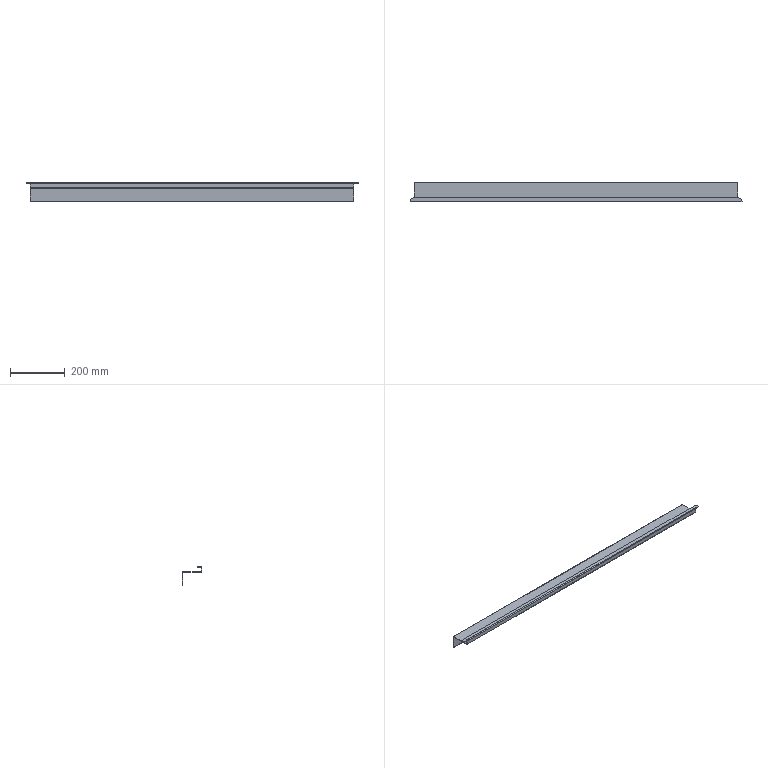Part | SolidWorks | features BaseBody 1 | 1 solid | 36 faces | box 1216 x 72 x 68 mm | volume 352774 mm3 | plane 24 | cylinder 8 | torus 4 | commonest cylinder face diameters 2 x3 6 x3 30 x2
STEP:
#1=CARTESIAN_POINT('',(596.,-36.,18.));
#2=VERTEX_POINT('',#1);
#3=CARTESIAN_POINT('',(593.,-36.,15.));
#4=VERTEX_POINT('',#3);
#5=CARTESIAN_POINT('',(596.,-36.,15.));
#6=DIRECTION('',(0.,-1.,0.));
#7=DIRECTION('',(0.,0.,1.));
#8=AXIS2_PLACEMENT_3D('',#5,#6,#7);
#9=CIRCLE('',#8,3.);
#10=EDGE_CURVE('',#2,#4,#9,.T.);
#11=ORIENTED_EDGE('',*,*,#10,.T.);
#12=CARTESIAN_POINT('',(595.,-36.,15.));
#13=VERTEX_POINT('',#12);
#14=CARTESIAN_POINT('',(595.,-36.,15.));
#15=DIRECTION('',(1.,0.,0.));
#16=VECTOR('',#15,1000.);
#17=LINE('',#14,#16);
#18=EDGE_CURVE('',#4,#13,#17,.T.);
#19=ORIENTED_EDGE('',*,*,#18,.T.);
#20=CARTESIAN_POINT('',(596.,-36.,16.));
#21=VERTEX_POINT('',#20);
#22=CARTESIAN_POINT('',(596.,-36.,15.));
#23=DIRECTION('',(0.,1.,0.));
#24=DIRECTION('',(0.,0.,1.));
#25=AXIS2_PLACEMENT_3D('',#22,#23,#24);
#26=CIRCLE('',#25,1.);
#27=EDGE_CURVE('',#13,#21,#26,.T.);
#28=ORIENTED_EDGE('',*,*,#27,.T.);
#29=CARTESIAN_POINT('',(608.,-36.,16.));
#30=VERTEX_POINT('',#29);
#31=CARTESIAN_POINT('',(608.,-36.,16.));
#32=DIRECTION('',(1.,0.,0.));
#33=VECTOR('',#32,1000.);
#34=LINE('',#31,#33);
#35=EDGE_CURVE('',#21,#30,#34,.T.);
#36=ORIENTED_EDGE('',*,*,#35,.T.);
#37=CARTESIAN_POINT('',(608.,-36.,18.));
#38=VERTEX_POINT('',#37);
#39=CARTESIAN_POINT('',(608.,-36.,18.));
#40=DIRECTION('',(0.,0.,1.));
#41=VECTOR('',#40,1000.);
#42=LINE('',#39,#41);
#43=EDGE_CURVE('',#30,#38,#42,.T.);
#44=ORIENTED_EDGE('',*,*,#43,.T.);
#45=CARTESIAN_POINT('',(596.,-36.,18.));
#46=DIRECTION('',(-1.,0.,0.));
#47=VECTOR('',#46,1000.);
#48=LINE('',#45,#47);
#49=EDGE_CURVE('',#38,#2,#48,.T.);
#50=ORIENTED_EDGE('',*,*,#49,.T.);
#51=EDGE_LOOP('',(#11,#19,#28,#36,#44,#50));
#52=FACE_OUTER_BOUND('',#51,.T.);
#53=CARTESIAN_POINT('',(596.,-36.,15.));
#54=DIRECTION('',(0.,-1.,0.));
#55=DIRECTION('',(0.,0.,-1.));
#56=AXIS2_PLACEMENT_3D('',#53,#54,#55);
#57=PLANE('',#56);
#58=ADVANCED_FACE('',(#52),#57,.T.);
#59=CARTESIAN_POINT('',(593.,-33.,16.));
#60=VERTEX_POINT('',#59);
#61=CARTESIAN_POINT('',(593.,-36.,16.));
#62=DIRECTION('',(0.,0.,-1.));
#63=DIRECTION('',(0.,1.,0.));
#64=AXIS2_PLACEMENT_3D('',#61,#62,#63);
#65=CIRCLE('',#64,3.);
#66=EDGE_CURVE('',#60,#21,#65,.T.);
#67=ORIENTED_EDGE('',*,*,#66,.T.);
#68=ORIENTED_EDGE('',*,*,#27,.F.);
#69=CARTESIAN_POINT('',(593.,-34.,15.));
#70=VERTEX_POINT('',#69);
#71=CARTESIAN_POINT('',(593.,-36.,15.));
#72=DIRECTION('',(0.,0.,-1.));
#73=DIRECTION('',(0.,1.,0.));
#74=AXIS2_PLACEMENT_3D('',#71,#72,#73);
#75=CIRCLE('',#74,2.);
#76=EDGE_CURVE('',#70,#13,#75,.T.);
#77=ORIENTED_EDGE('',*,*,#76,.F.);
#78=CARTESIAN_POINT('',(593.,-33.,15.));
#79=DIRECTION('',(1.,0.,0.));
#80=DIRECTION('',(0.,0.,-1.));
#81=AXIS2_PLACEMENT_3D('',#78,#79,#80);
#82=CIRCLE('',#81,1.);
#83=EDGE_CURVE('',#60,#70,#82,.T.);
#84=ORIENTED_EDGE('',*,*,#83,.F.);
#85=EDGE_LOOP('',(#67,#68,#77,#84));
#86=FACE_OUTER_BOUND('',#85,.T.);
#87=CARTESIAN_POINT('',(593.,-36.,15.));
#88=DIRECTION('',(0.,0.,-1.));
#89=DIRECTION('',(-1.,0.,0.));
#90=AXIS2_PLACEMENT_3D('',#87,#88,#89);
#91=TOROIDAL_SURFACE('',#90,3.,1.);
#92=ADVANCED_FACE('',(#86),#91,.F.);
#93=CARTESIAN_POINT('',(593.,-21.,18.));
#94=VERTEX_POINT('',#93);
#95=CARTESIAN_POINT('',(593.,-36.,18.));
#96=DIRECTION('',(0.,0.,-1.));
#97=DIRECTION('',(0.,1.,0.));
#98=AXIS2_PLACEMENT_3D('',#95,#96,#97);
#99=CIRCLE('',#98,15.);
#100=EDGE_CURVE('',#94,#38,#99,.T.);
#101=ORIENTED_EDGE('',*,*,#100,.T.);
#102=ORIENTED_EDGE('',*,*,#43,.F.);
#103=CARTESIAN_POINT('',(593.,-21.,16.));
#104=VERTEX_POINT('',#103);
#105=CARTESIAN_POINT('',(593.,-36.,16.));
#106=DIRECTION('',(0.,0.,-1.));
#107=DIRECTION('',(0.,1.,0.));
#108=AXIS2_PLACEMENT_3D('',#105,#106,#107);
#109=CIRCLE('',#108,15.);
#110=EDGE_CURVE('',#104,#30,#109,.T.);
#111=ORIENTED_EDGE('',*,*,#110,.F.);
#112=CARTESIAN_POINT('',(593.,-21.,18.));
#113=DIRECTION('',(0.,0.,-1.));
#114=VECTOR('',#113,1000.);
#115=LINE('',#112,#114);
#116=EDGE_CURVE('',#94,#104,#115,.T.);
#117=ORIENTED_EDGE('',*,*,#116,.F.);
#118=EDGE_LOOP('',(#101,#102,#111,#117));
#119=FACE_OUTER_BOUND('',#118,.T.);
#120=CARTESIAN_POINT('',(593.,-36.,18.));
#121=DIRECTION('',(0.,0.,-1.));
#122=DIRECTION('',(-1.,0.,0.));
#123=AXIS2_PLACEMENT_3D('',#120,#121,#122);
#124=CYLINDRICAL_SURFACE('',#123,15.);
#125=ADVANCED_FACE('',(#119),#124,.T.);
#126=CARTESIAN_POINT('',(593.,-33.,18.));
#127=VERTEX_POINT('',#126);
#128=CARTESIAN_POINT('',(593.,-33.,15.));
#129=DIRECTION('',(1.,0.,0.));
#130=DIRECTION('',(0.,0.,-1.));
#131=AXIS2_PLACEMENT_3D('',#128,#129,#130);
#132=CIRCLE('',#131,3.);
#133=EDGE_CURVE('',#127,#4,#132,.T.);
#134=ORIENTED_EDGE('',*,*,#133,.T.);
#135=ORIENTED_EDGE('',*,*,#10,.F.);
#136=CARTESIAN_POINT('',(593.,-36.,18.));
#137=DIRECTION('',(0.,0.,-1.));
#138=DIRECTION('',(0.,1.,0.));
#139=AXIS2_PLACEMENT_3D('',#136,#137,#138);
#140=CIRCLE('',#139,3.);
#141=EDGE_CURVE('',#127,#2,#140,.T.);
#142=ORIENTED_EDGE('',*,*,#141,.F.);
#143=EDGE_LOOP('',(#134,#135,#142));
#144=FACE_OUTER_BOUND('',#143,.T.);
#145=CARTESIAN_POINT('',(593.,-36.,15.));
#146=DIRECTION('',(0.,0.,-1.));
#147=DIRECTION('',(-1.,0.,0.));
#148=AXIS2_PLACEMENT_3D('',#145,#146,#147);
#149=TOROIDAL_SURFACE('',#148,3.,3.);
#150=ADVANCED_FACE('',(#144),#149,.T.);
#151=ORIENTED_EDGE('',*,*,#18,.F.);
#152=CARTESIAN_POINT('',(593.,-34.,15.));
#153=DIRECTION('',(0.,-1.,0.));
#154=VECTOR('',#153,1000.);
#155=LINE('',#152,#154);
#156=EDGE_CURVE('',#70,#4,#155,.T.);
#157=ORIENTED_EDGE('',*,*,#156,.F.);
#158=ORIENTED_EDGE('',*,*,#76,.T.);
#159=EDGE_LOOP('',(#151,#157,#158));
#160=FACE_OUTER_BOUND('',#159,.T.);
#161=CARTESIAN_POINT('',(593.,-34.,15.));
#162=DIRECTION('',(0.,0.,-1.));
#163=DIRECTION('',(0.,-1.,0.));
#164=AXIS2_PLACEMENT_3D('',#161,#162,#163);
#165=PLANE('',#164);
#166=ADVANCED_FACE('',(#160),#165,.T.);
#167=CARTESIAN_POINT('',(-593.,-36.,15.));
#168=VERTEX_POINT('',#167);
#169=CARTESIAN_POINT('',(-596.,-36.,18.));
#170=VERTEX_POINT('',#169);
#171=CARTESIAN_POINT('',(-596.,-36.,15.));
#172=DIRECTION('',(0.,-1.,0.));
#173=DIRECTION('',(0.,0.,1.));
#174=AXIS2_PLACEMENT_3D('',#171,#172,#173);
#175=CIRCLE('',#174,3.);
#176=EDGE_CURVE('',#168,#170,#175,.T.);
#177=ORIENTED_EDGE('',*,*,#176,.T.);
#178=CARTESIAN_POINT('',(-608.,-36.,18.));
#179=VERTEX_POINT('',#178);
#180=CARTESIAN_POINT('',(-596.,-36.,18.));
#181=DIRECTION('',(-1.,0.,0.));
#182=VECTOR('',#181,1000.);
#183=LINE('',#180,#182);
#184=EDGE_CURVE('',#170,#179,#183,.T.);
#185=ORIENTED_EDGE('',*,*,#184,.T.);
#186=CARTESIAN_POINT('',(-608.,-36.,16.));
#187=VERTEX_POINT('',#186);
#188=CARTESIAN_POINT('',(-608.,-36.,18.));
#189=DIRECTION('',(0.,0.,-1.));
#190=VECTOR('',#189,1000.);
#191=LINE('',#188,#190);
#192=EDGE_CURVE('',#179,#187,#191,.T.);
#193=ORIENTED_EDGE('',*,*,#192,.T.);
#194=CARTESIAN_POINT('',(-596.,-36.,16.));
#195=VERTEX_POINT('',#194);
#196=CARTESIAN_POINT('',(-608.,-36.,16.));
#197=DIRECTION('',(1.,0.,0.));
#198=VECTOR('',#197,1000.);
#199=LINE('',#196,#198);
#200=EDGE_CURVE('',#187,#195,#199,.T.);
#201=ORIENTED_EDGE('',*,*,#200,.T.);
#202=CARTESIAN_POINT('',(-595.,-36.,15.));
#203=VERTEX_POINT('',#202);
#204=CARTESIAN_POINT('',(-596.,-36.,15.));
#205=DIRECTION('',(0.,1.,0.));
#206=DIRECTION('',(0.,0.,1.));
#207=AXIS2_PLACEMENT_3D('',#204,#205,#206);
#208=CIRCLE('',#207,1.);
#209=EDGE_CURVE('',#195,#203,#208,.T.);
#210=ORIENTED_EDGE('',*,*,#209,.T.);
#211=CARTESIAN_POINT('',(-595.,-36.,15.));
#212=DIRECTION('',(1.,0.,0.));
#213=VECTOR('',#212,1000.);
#214=LINE('',#211,#213);
#215=EDGE_CURVE('',#203,#168,#214,.T.);
#216=ORIENTED_EDGE('',*,*,#215,.T.);
#217=EDGE_LOOP('',(#177,#185,#193,#201,#210,#216));
#218=FACE_OUTER_BOUND('',#217,.T.);
#219=CARTESIAN_POINT('',(-596.,-36.,15.));
#220=DIRECTION('',(0.,-1.,0.));
#221=DIRECTION('',(0.,0.,-1.));
#222=AXIS2_PLACEMENT_3D('',#219,#220,#221);
#223=PLANE('',#222);
#224=ADVANCED_FACE('',(#218),#223,.T.);
#225=CARTESIAN_POINT('',(-593.,-33.,18.));
#226=VERTEX_POINT('',#225);
#227=CARTESIAN_POINT('',(-593.,-36.,18.));
#228=DIRECTION('',(0.,0.,1.));
#229=DIRECTION('',(0.,1.,0.));
#230=AXIS2_PLACEMENT_3D('',#227,#228,#229);
#231=CIRCLE('',#230,3.);
#232=EDGE_CURVE('',#226,#170,#231,.T.);
#233=ORIENTED_EDGE('',*,*,#232,.T.);
#234=ORIENTED_EDGE('',*,*,#176,.F.);
#235=CARTESIAN_POINT('',(-593.,-33.,15.));
#236=DIRECTION('',(-1.,0.,0.));
#237=DIRECTION('',(0.,0.,-1.));
#238=AXIS2_PLACEMENT_3D('',#235,#236,#237);
#239=CIRCLE('',#238,3.);
#240=EDGE_CURVE('',#168,#226,#239,.T.);
#241=ORIENTED_EDGE('',*,*,#240,.T.);
#242=EDGE_LOOP('',(#233,#234,#241));
#243=FACE_OUTER_BOUND('',#242,.T.);
#244=CARTESIAN_POINT('',(-593.,-36.,15.));
#245=DIRECTION('',(0.,0.,1.));
#246=DIRECTION('',(1.,0.,0.));
#247=AXIS2_PLACEMENT_3D('',#244,#245,#246);
#248=TOROIDAL_SURFACE('',#247,3.,3.);
#249=ADVANCED_FACE('',(#243),#248,.T.);
#250=CARTESIAN_POINT('',(-593.,-21.,16.));
#251=VERTEX_POINT('',#250);
#252=CARTESIAN_POINT('',(-593.,-36.,16.));
#253=DIRECTION('',(0.,0.,1.));
#254=DIRECTION('',(0.,1.,0.));
#255=AXIS2_PLACEMENT_3D('',#252,#253,#254);
#256=CIRCLE('',#255,15.);
#257=EDGE_CURVE('',#251,#187,#256,.T.);
#258=ORIENTED_EDGE('',*,*,#257,.T.);
#259=ORIENTED_EDGE('',*,*,#192,.F.);
#260=CARTESIAN_POINT('',(-593.,-21.,18.));
#261=VERTEX_POINT('',#260);
#262=CARTESIAN_POINT('',(-593.,-36.,18.));
#263=DIRECTION('',(0.,0.,1.));
#264=DIRECTION('',(0.,1.,0.));
#265=AXIS2_PLACEMENT_3D('',#262,#263,#264);
#266=CIRCLE('',#265,15.);
#267=EDGE_CURVE('',#261,#179,#266,.T.);
#268=ORIENTED_EDGE('',*,*,#267,.F.);
#269=CARTESIAN_POINT('',(-593.,-21.,18.));
#270=DIRECTION('',(0.,0.,-1.));
#271=VECTOR('',#270,1000.);
#272=LINE('',#269,#271);
#273=EDGE_CURVE('',#261,#251,#272,.T.);
#274=ORIENTED_EDGE('',*,*,#273,.T.);
#275=EDGE_LOOP('',(#258,#259,#268,#274));
#276=FACE_OUTER_BOUND('',#275,.T.);
#277=CARTESIAN_POINT('',(-593.,-36.,18.));
#278=DIRECTION('',(0.,0.,1.));
#279=DIRECTION('',(1.,0.,0.));
#280=AXIS2_PLACEMENT_3D('',#277,#278,#279);
#281=CYLINDRICAL_SURFACE('',#280,15.);
#282=ADVANCED_FACE('',(#276),#281,.T.);
#283=CARTESIAN_POINT('',(-593.,-34.,15.));
#284=VERTEX_POINT('',#283);
#285=CARTESIAN_POINT('',(-593.,-36.,15.));
#286=DIRECTION('',(0.,0.,1.));
#287=DIRECTION('',(0.,1.,0.));
#288=AXIS2_PLACEMENT_3D('',#285,#286,#287);
#289=CIRCLE('',#288,2.);
#290=EDGE_CURVE('',#284,#203,#289,.T.);
#291=ORIENTED_EDGE('',*,*,#290,.T.);
#292=ORIENTED_EDGE('',*,*,#209,.F.);
#293=CARTESIAN_POINT('',(-593.,-33.,16.));
#294=VERTEX_POINT('',#293);
#295=CARTESIAN_POINT('',(-593.,-36.,16.));
#296=DIRECTION('',(0.,0.,1.));
#297=DIRECTION('',(0.,1.,0.));
#298=AXIS2_PLACEMENT_3D('',#295,#296,#297);
#299=CIRCLE('',#298,3.);
#300=EDGE_CURVE('',#294,#195,#299,.T.);
#301=ORIENTED_EDGE('',*,*,#300,.F.);
#302=CARTESIAN_POINT('',(-593.,-33.,15.));
#303=DIRECTION('',(-1.,0.,0.));
#304=DIRECTION('',(0.,0.,-1.));
#305=AXIS2_PLACEMENT_3D('',#302,#303,#304);
#306=CIRCLE('',#305,1.);
#307=EDGE_CURVE('',#284,#294,#306,.T.);
#308=ORIENTED_EDGE('',*,*,#307,.F.);
#309=EDGE_LOOP('',(#291,#292,#301,#308));
#310=FACE_OUTER_BOUND('',#309,.T.);
#311=CARTESIAN_POINT('',(-593.,-36.,15.));
#312=DIRECTION('',(0.,0.,1.));
#313=DIRECTION('',(1.,0.,0.));
#314=AXIS2_PLACEMENT_3D('',#311,#312,#313);
#315=TOROIDAL_SURFACE('',#314,3.,1.);
#316=ADVANCED_FACE('',(#310),#315,.F.);
#317=ORIENTED_EDGE('',*,*,#215,.F.);
#318=ORIENTED_EDGE('',*,*,#290,.F.);
#319=CARTESIAN_POINT('',(-593.,-34.,15.));
#320=DIRECTION('',(0.,-1.,0.));
#321=VECTOR('',#320,1000.);
#322=LINE('',#319,#321);
#323=EDGE_CURVE('',#284,#168,#322,.T.);
#324=ORIENTED_EDGE('',*,*,#323,.T.);
#325=EDGE_LOOP('',(#317,#318,#324));
#326=FACE_OUTER_BOUND('',#325,.T.);
#327=CARTESIAN_POINT('',(-593.,-34.,15.));
#328=DIRECTION('',(0.,0.,-1.));
#329=DIRECTION('',(0.,-1.,0.));
#330=AXIS2_PLACEMENT_3D('',#327,#328,#329);
#331=PLANE('',#330);
#332=ADVANCED_FACE('',(#326),#331,.T.);
#333=CARTESIAN_POINT('',(-593.,-21.,16.));
#334=DIRECTION('',(-1.,0.,0.));
#335=VECTOR('',#334,1000.);
#336=LINE('',#333,#335);
#337=EDGE_CURVE('',#104,#251,#336,.T.);
#338=ORIENTED_EDGE('',*,*,#337,.T.);
#339=ORIENTED_EDGE('',*,*,#273,.F.);
#340=CARTESIAN_POINT('',(0.,-21.,18.));
#341=DIRECTION('',(-1.,0.,0.));
#342=VECTOR('',#341,1000.);
#343=LINE('',#340,#342);
#344=EDGE_CURVE('',#94,#261,#343,.T.);
#345=ORIENTED_EDGE('',*,*,#344,.F.);
#346=ORIENTED_EDGE('',*,*,#116,.T.);
#347=EDGE_LOOP('',(#338,#339,#345,#346));
#348=FACE_OUTER_BOUND('',#347,.T.);
#349=CARTESIAN_POINT('',(-593.,-21.,18.));
#350=DIRECTION('',(0.,-1.,0.));
#351=DIRECTION('',(0.,0.,-1.));
#352=AXIS2_PLACEMENT_3D('',#349,#350,#351);
#353=PLANE('',#352);
#354=ADVANCED_FACE('',(#348),#353,.F.);
#355=ORIENTED_EDGE('',*,*,#337,.F.);
#356=ORIENTED_EDGE('',*,*,#110,.T.);
#357=ORIENTED_EDGE('',*,*,#35,.F.);
#358=ORIENTED_EDGE('',*,*,#66,.F.);
#359=CARTESIAN_POINT('',(-593.,-33.,16.));
#360=DIRECTION('',(1.,0.,0.));
#361=VECTOR('',#360,1000.);
#362=LINE('',#359,#361);
#363=EDGE_CURVE('',#294,#60,#362,.T.);
#364=ORIENTED_EDGE('',*,*,#363,.F.);
#365=ORIENTED_EDGE('',*,*,#300,.T.);
#366=ORIENTED_EDGE('',*,*,#200,.F.);
#367=ORIENTED_EDGE('',*,*,#257,.F.);
#368=EDGE_LOOP('',(#355,#356,#357,#358,#364,#365,#366,#367));
#369=FACE_OUTER_BOUND('',#368,.T.);
#370=CARTESIAN_POINT('',(0.,0.,16.));
#371=DIRECTION('',(0.,0.,-1.));
#372=DIRECTION('',(0.,-1.,0.));
#373=AXIS2_PLACEMENT_3D('',#370,#371,#372);
#374=PLANE('',#373);
#375=ADVANCED_FACE('',(#369),#374,.T.);
#376=CARTESIAN_POINT('',(-593.,-33.,18.));
#377=DIRECTION('',(-1.,0.,0.));
#378=VECTOR('',#377,1000.);
#379=LINE('',#376,#378);
#380=EDGE_CURVE('',#127,#226,#379,.T.);
#381=ORIENTED_EDGE('',*,*,#380,.F.);
#382=ORIENTED_EDGE('',*,*,#141,.T.);
#383=ORIENTED_EDGE('',*,*,#49,.F.);
#384=ORIENTED_EDGE('',*,*,#100,.F.);
#385=ORIENTED_EDGE('',*,*,#344,.T.);
#386=ORIENTED_EDGE('',*,*,#267,.T.);
#387=ORIENTED_EDGE('',*,*,#184,.F.);
#388=ORIENTED_EDGE('',*,*,#232,.F.);
#389=EDGE_LOOP('',(#381,#382,#383,#384,#385,#386,#387,#388));
#390=FACE_OUTER_BOUND('',#389,.T.);
#391=CARTESIAN_POINT('',(0.,0.,18.));
#392=DIRECTION('',(0.,0.,-1.));
#393=DIRECTION('',(0.,-1.,0.));
#394=AXIS2_PLACEMENT_3D('',#391,#392,#393);
#395=PLANE('',#394);
#396=ADVANCED_FACE('',(#390),#395,.F.);
#397=CARTESIAN_POINT('',(593.,-34.,15.));
#398=DIRECTION('',(-1.,0.,0.));
#399=VECTOR('',#398,1000.);
#400=LINE('',#397,#399);
#401=EDGE_CURVE('',#70,#284,#400,.T.);
#402=ORIENTED_EDGE('',*,*,#401,.T.);
#403=ORIENTED_EDGE('',*,*,#307,.T.);
#404=ORIENTED_EDGE('',*,*,#363,.T.);
#405=ORIENTED_EDGE('',*,*,#83,.T.);
#406=EDGE_LOOP('',(#402,#403,#404,#405));
#407=FACE_OUTER_BOUND('',#406,.T.);
#408=CARTESIAN_POINT('',(593.,-33.,15.));
#409=DIRECTION('',(1.,0.,0.));
#410=DIRECTION('',(0.,0.,1.));
#411=AXIS2_PLACEMENT_3D('',#408,#409,#410);
#412=CYLINDRICAL_SURFACE('',#411,1.);
#413=ADVANCED_FACE('',(#407),#412,.F.);
#414=CARTESIAN_POINT('',(593.,-36.,15.));
#415=DIRECTION('',(-1.,0.,0.));
#416=VECTOR('',#415,1000.);
#417=LINE('',#414,#416);
#418=EDGE_CURVE('',#4,#168,#417,.T.);
#419=ORIENTED_EDGE('',*,*,#418,.F.);
#420=ORIENTED_EDGE('',*,*,#133,.F.);
#421=ORIENTED_EDGE('',*,*,#380,.T.);
#422=ORIENTED_EDGE('',*,*,#240,.F.);
#423=EDGE_LOOP('',(#419,#420,#421,#422));
#424=FACE_OUTER_BOUND('',#423,.T.);
#425=CARTESIAN_POINT('',(593.,-33.,15.));
#426=DIRECTION('',(1.,0.,0.));
#427=DIRECTION('',(0.,0.,1.));
#428=AXIS2_PLACEMENT_3D('',#425,#426,#427);
#429=CYLINDRICAL_SURFACE('',#428,3.);
#430=ADVANCED_FACE('',(#424),#429,.T.);
#431=CARTESIAN_POINT('',(593.,-33.,0.));
#432=VERTEX_POINT('',#431);
#433=CARTESIAN_POINT('',(-593.,-33.,0.));
#434=VERTEX_POINT('',#433);
#435=CARTESIAN_POINT('',(593.,-33.,0.));
#436=DIRECTION('',(-1.,0.,0.));
#437=VECTOR('',#436,1000.);
#438=LINE('',#435,#437);
#439=EDGE_CURVE('',#432,#434,#438,.T.);
#440=ORIENTED_EDGE('',*,*,#439,.T.);
#441=CARTESIAN_POINT('',(-593.,-34.,1.));
#442=VERTEX_POINT('',#441);
#443=CARTESIAN_POINT('',(-593.,-33.,1.));
#444=DIRECTION('',(-1.,0.,0.));
#445=DIRECTION('',(0.,0.,-1.));
#446=AXIS2_PLACEMENT_3D('',#443,#444,#445);
#447=CIRCLE('',#446,1.);
#448=EDGE_CURVE('',#434,#442,#447,.T.);
#449=ORIENTED_EDGE('',*,*,#448,.T.);
#450=CARTESIAN_POINT('',(593.,-34.,1.));
#451=VERTEX_POINT('',#450);
#452=CARTESIAN_POINT('',(-593.,-34.,1.));
#453=DIRECTION('',(1.,0.,0.));
#454=VECTOR('',#453,1000.);
#455=LINE('',#452,#454);
#456=EDGE_CURVE('',#442,#451,#455,.T.);
#457=ORIENTED_EDGE('',*,*,#456,.T.);
#458=CARTESIAN_POINT('',(593.,-33.,1.));
#459=DIRECTION('',(1.,0.,0.));
#460=DIRECTION('',(0.,0.,-1.));
#461=AXIS2_PLACEMENT_3D('',#458,#459,#460);
#462=CIRCLE('',#461,1.);
#463=EDGE_CURVE('',#451,#432,#462,.T.);
#464=ORIENTED_EDGE('',*,*,#463,.T.);
#465=EDGE_LOOP('',(#440,#449,#457,#464));
#466=FACE_OUTER_BOUND('',#465,.T.);
#467=CARTESIAN_POINT('',(593.,-33.,1.));
#468=DIRECTION('',(1.,0.,0.));
#469=DIRECTION('',(0.,-1.,0.));
#470=AXIS2_PLACEMENT_3D('',#467,#468,#469);
#471=CYLINDRICAL_SURFACE('',#470,1.);
#472=ADVANCED_FACE('',(#466),#471,.F.);
#473=CARTESIAN_POINT('',(593.,-33.,-2.));
#474=VERTEX_POINT('',#473);
#475=CARTESIAN_POINT('',(-593.,-33.,-2.));
#476=VERTEX_POINT('',#475);
#477=CARTESIAN_POINT('',(593.,-33.,-2.));
#478=DIRECTION('',(-1.,0.,0.));
#479=VECTOR('',#478,1000.);
#480=LINE('',#477,#479);
#481=EDGE_CURVE('',#474,#476,#480,.T.);
#482=ORIENTED_EDGE('',*,*,#481,.F.);
#483=CARTESIAN_POINT('',(593.,-36.,1.));
#484=VERTEX_POINT('',#483);
#485=CARTESIAN_POINT('',(593.,-33.,1.));
#486=DIRECTION('',(1.,0.,0.));
#487=DIRECTION('',(0.,0.,-1.));
#488=AXIS2_PLACEMENT_3D('',#485,#486,#487);
#489=CIRCLE('',#488,3.);
#490=EDGE_CURVE('',#484,#474,#489,.T.);
#491=ORIENTED_EDGE('',*,*,#490,.F.);
#492=CARTESIAN_POINT('',(-593.,-36.,1.));
#493=VERTEX_POINT('',#492);
#494=CARTESIAN_POINT('',(-593.,-36.,1.));
#495=DIRECTION('',(-1.,0.,0.));
#496=VECTOR('',#495,1000.);
#497=LINE('',#494,#496);
#498=EDGE_CURVE('',#484,#493,#497,.T.);
#499=ORIENTED_EDGE('',*,*,#498,.T.);
#500=CARTESIAN_POINT('',(-593.,-33.,1.));
#501=DIRECTION('',(-1.,0.,0.));
#502=DIRECTION('',(0.,0.,-1.));
#503=AXIS2_PLACEMENT_3D('',#500,#501,#502);
#504=CIRCLE('',#503,3.);
#505=EDGE_CURVE('',#476,#493,#504,.T.);
#506=ORIENTED_EDGE('',*,*,#505,.F.);
#507=EDGE_LOOP('',(#482,#491,#499,#506));
#508=FACE_OUTER_BOUND('',#507,.T.);
#509=CARTESIAN_POINT('',(593.,-33.,1.));
#510=DIRECTION('',(1.,0.,0.));
#511=DIRECTION('',(0.,-1.,0.));
#512=AXIS2_PLACEMENT_3D('',#509,#510,#511);
#513=CYLINDRICAL_SURFACE('',#512,3.);
#514=ADVANCED_FACE('',(#508),#513,.T.);
#515=ORIENTED_EDGE('',*,*,#463,.F.);
#516=CARTESIAN_POINT('',(593.,-34.,1.));
#517=DIRECTION('',(0.,-1.,0.));
#518=VECTOR('',#517,1000.);
#519=LINE('',#516,#518);
#520=EDGE_CURVE('',#451,#484,#519,.T.);
#521=ORIENTED_EDGE('',*,*,#520,.T.);
#522=ORIENTED_EDGE('',*,*,#490,.T.);
#523=CARTESIAN_POINT('',(593.,-33.,0.));
#524=DIRECTION('',(0.,0.,-1.));
#525=VECTOR('',#524,1000.);
#526=LINE('',#523,#525);
#527=EDGE_CURVE('',#432,#474,#526,.T.);
#528=ORIENTED_EDGE('',*,*,#527,.F.);
#529=EDGE_LOOP('',(#515,#521,#522,#528));
#530=FACE_OUTER_BOUND('',#529,.T.);
#531=CARTESIAN_POINT('',(593.,-33.,1.));
#532=DIRECTION('',(-1.,0.,0.));
#533=DIRECTION('',(0.,0.,1.));
#534=AXIS2_PLACEMENT_3D('',#531,#532,#533);
#535=PLANE('',#534);
#536=ADVANCED_FACE('',(#530),#535,.F.);
#537=CARTESIAN_POINT('',(-593.,-36.,1.));
#538=DIRECTION('',(0.,-1.,0.));
#539=VECTOR('',#538,1000.);
#540=LINE('',#537,#539);
#541=EDGE_CURVE('',#442,#493,#540,.T.);
#542=ORIENTED_EDGE('',*,*,#541,.F.);
#543=ORIENTED_EDGE('',*,*,#448,.F.);
#544=CARTESIAN_POINT('',(-593.,-33.,0.));
#545=DIRECTION('',(0.,0.,-1.));
#546=VECTOR('',#545,1000.);
#547=LINE('',#544,#546);
#548=EDGE_CURVE('',#434,#476,#547,.T.);
#549=ORIENTED_EDGE('',*,*,#548,.T.);
#550=ORIENTED_EDGE('',*,*,#505,.T.);
#551=EDGE_LOOP('',(#542,#543,#549,#550));
#552=FACE_OUTER_BOUND('',#551,.T.);
#553=CARTESIAN_POINT('',(-593.,-33.,1.));
#554=DIRECTION('',(-1.,0.,0.));
#555=DIRECTION('',(0.,0.,1.));
#556=AXIS2_PLACEMENT_3D('',#553,#554,#555);
#557=PLANE('',#556);
#558=ADVANCED_FACE('',(#552),#557,.T.);
#559=CARTESIAN_POINT('',(-593.,34.,-50.));
#560=VERTEX_POINT('',#559);
#561=CARTESIAN_POINT('',(593.,34.,-50.));
#562=VERTEX_POINT('',#561);
#563=CARTESIAN_POINT('',(0.,34.,-50.));
#564=DIRECTION('',(1.,0.,0.));
#565=VECTOR('',#564,1000.);
#566=LINE('',#563,#565);
#567=EDGE_CURVE('',#560,#562,#566,.T.);
#568=ORIENTED_EDGE('',*,*,#567,.F.);
#569=CARTESIAN_POINT('',(-593.,36.,-50.));
#570=VERTEX_POINT('',#569);
#571=CARTESIAN_POINT('',(-593.,36.,-50.));
#572=DIRECTION('',(0.,-1.,0.));
#573=VECTOR('',#572,1000.);
#574=LINE('',#571,#573);
#575=EDGE_CURVE('',#570,#560,#574,.T.);
#576=ORIENTED_EDGE('',*,*,#575,.F.);
#577=CARTESIAN_POINT('',(593.,36.,-50.));
#578=VERTEX_POINT('',#577);
#579=CARTESIAN_POINT('',(593.,36.,-50.));
#580=DIRECTION('',(1.,0.,0.));
#581=VECTOR('',#580,1000.);
#582=LINE('',#579,#581);
#583=EDGE_CURVE('',#570,#578,#582,.T.);
#584=ORIENTED_EDGE('',*,*,#583,.T.);
#585=CARTESIAN_POINT('',(593.,36.,-50.));
#586=DIRECTION('',(0.,-1.,0.));
#587=VECTOR('',#586,1000.);
#588=LINE('',#585,#587);
#589=EDGE_CURVE('',#578,#562,#588,.T.);
#590=ORIENTED_EDGE('',*,*,#589,.T.);
#591=EDGE_LOOP('',(#568,#576,#584,#590));
#592=FACE_OUTER_BOUND('',#591,.T.);
#593=CARTESIAN_POINT('',(593.,36.,-50.));
#594=DIRECTION('',(0.,0.,-1.));
#595=DIRECTION('',(-1.,0.,0.));
#596=AXIS2_PLACEMENT_3D('',#593,#594,#595);
#597=PLANE('',#596);
#598=ADVANCED_FACE('',(#592),#597,.T.);
#599=CARTESIAN_POINT('',(-593.,34.,-3.));
#600=VERTEX_POINT('',#599);
#601=CARTESIAN_POINT('',(593.,34.,-3.));
#602=VERTEX_POINT('',#601);
#603=CARTESIAN_POINT('',(-593.,34.,-3.));
#604=DIRECTION('',(1.,0.,0.));
#605=VECTOR('',#604,1000.);
#606=LINE('',#603,#605);
#607=EDGE_CURVE('',#600,#602,#606,.T.);
#608=ORIENTED_EDGE('',*,*,#607,.F.);
#609=CARTESIAN_POINT('',(-593.,34.,0.));
#610=DIRECTION('',(0.,0.,-1.));
#611=VECTOR('',#610,1000.);
#612=LINE('',#609,#611);
#613=EDGE_CURVE('',#600,#560,#612,.T.);
#614=ORIENTED_EDGE('',*,*,#613,.T.);
#615=ORIENTED_EDGE('',*,*,#567,.T.);
#616=CARTESIAN_POINT('',(593.,34.,0.));
#617=DIRECTION('',(0.,0.,1.));
#618=VECTOR('',#617,1000.);
#619=LINE('',#616,#618);
#620=EDGE_CURVE('',#562,#602,#619,.T.);
#621=ORIENTED_EDGE('',*,*,#620,.T.);
#622=EDGE_LOOP('',(#608,#614,#615,#621));
#623=FACE_OUTER_BOUND('',#622,.T.);
#624=CARTESIAN_POINT('',(0.,34.,0.));
#625=DIRECTION('',(0.,1.,0.));
#626=DIRECTION('',(0.,0.,-1.));
#627=AXIS2_PLACEMENT_3D('',#624,#625,#626);
#628=PLANE('',#627);
#629=ADVANCED_FACE('',(#623),#628,.F.);
#630=CARTESIAN_POINT('',(-593.,36.,-3.));
#631=VERTEX_POINT('',#630);
#632=CARTESIAN_POINT('',(-593.,36.,-50.));
#633=DIRECTION('',(0.,0.,-1.));
#634=VECTOR('',#633,1000.);
#635=LINE('',#632,#634);
#636=EDGE_CURVE('',#631,#570,#635,.T.);
#637=ORIENTED_EDGE('',*,*,#636,.F.);
#638=CARTESIAN_POINT('',(593.,36.,-3.));
#639=VERTEX_POINT('',#638);
#640=CARTESIAN_POINT('',(0.,36.,-3.));
#641=DIRECTION('',(1.,0.,0.));
#642=VECTOR('',#641,1000.);
#643=LINE('',#640,#642);
#644=EDGE_CURVE('',#631,#639,#643,.T.);
#645=ORIENTED_EDGE('',*,*,#644,.T.);
#646=CARTESIAN_POINT('',(593.,36.,-2.));
#647=DIRECTION('',(0.,0.,1.));
#648=VECTOR('',#647,1000.);
#649=LINE('',#646,#648);
#650=EDGE_CURVE('',#578,#639,#649,.T.);
#651=ORIENTED_EDGE('',*,*,#650,.F.);
#652=ORIENTED_EDGE('',*,*,#583,.F.);
#653=EDGE_LOOP('',(#637,#645,#651,#652));
#654=FACE_OUTER_BOUND('',#653,.T.);
#655=CARTESIAN_POINT('',(0.,36.,0.));
#656=DIRECTION('',(0.,1.,0.));
#657=DIRECTION('',(0.,0.,-1.));
#658=AXIS2_PLACEMENT_3D('',#655,#656,#657);
#659=PLANE('',#658);
#660=ADVANCED_FACE('',(#654),#659,.T.);
#661=ORIENTED_EDGE('',*,*,#650,.T.);
#662=CARTESIAN_POINT('',(593.,34.,-3.));
#663=DIRECTION('',(0.,1.,0.));
#664=VECTOR('',#663,1000.);
#665=LINE('',#662,#664);
#666=EDGE_CURVE('',#602,#639,#665,.T.);
#667=ORIENTED_EDGE('',*,*,#666,.F.);
#668=ORIENTED_EDGE('',*,*,#620,.F.);
#669=ORIENTED_EDGE('',*,*,#589,.F.);
#670=EDGE_LOOP('',(#661,#667,#668,#669));
#671=FACE_OUTER_BOUND('',#670,.T.);
#672=CARTESIAN_POINT('',(593.,36.,-2.));
#673=DIRECTION('',(1.,0.,0.));
#674=DIRECTION('',(0.,1.,0.));
#675=AXIS2_PLACEMENT_3D('',#672,#673,#674);
#676=PLANE('',#675);
#677=ADVANCED_FACE('',(#671),#676,.T.);
#678=ORIENTED_EDGE('',*,*,#613,.F.);
#679=CARTESIAN_POINT('',(-593.,36.,-3.));
#680=DIRECTION('',(0.,1.,0.));
#681=VECTOR('',#680,1000.);
#682=LINE('',#679,#681);
#683=EDGE_CURVE('',#600,#631,#682,.T.);
#684=ORIENTED_EDGE('',*,*,#683,.T.);
#685=ORIENTED_EDGE('',*,*,#636,.T.);
#686=ORIENTED_EDGE('',*,*,#575,.T.);
#687=EDGE_LOOP('',(#678,#684,#685,#686));
#688=FACE_OUTER_BOUND('',#687,.T.);
#689=CARTESIAN_POINT('',(-593.,36.,-50.));
#690=DIRECTION('',(-1.,0.,0.));
#691=DIRECTION('',(0.,0.,1.));
#692=AXIS2_PLACEMENT_3D('',#689,#690,#691);
#693=PLANE('',#692);
#694=ADVANCED_FACE('',(#688),#693,.T.);
#695=CARTESIAN_POINT('',(593.,33.,-2.));
#696=VERTEX_POINT('',#695);
#697=CARTESIAN_POINT('',(-593.,33.,-2.));
#698=VERTEX_POINT('',#697);
#699=CARTESIAN_POINT('',(593.,33.,-2.));
#700=DIRECTION('',(-1.,0.,0.));
#701=VECTOR('',#700,1000.);
#702=LINE('',#699,#701);
#703=EDGE_CURVE('',#696,#698,#702,.T.);
#704=ORIENTED_EDGE('',*,*,#703,.T.);
#705=CARTESIAN_POINT('',(-593.,33.,-3.));
#706=DIRECTION('',(-1.,0.,0.));
#707=DIRECTION('',(0.,0.,-1.));
#708=AXIS2_PLACEMENT_3D('',#705,#706,#707);
#709=CIRCLE('',#708,1.);
#710=EDGE_CURVE('',#698,#600,#709,.T.);
#711=ORIENTED_EDGE('',*,*,#710,.T.);
#712=ORIENTED_EDGE('',*,*,#607,.T.);
#713=CARTESIAN_POINT('',(593.,33.,-3.));
#714=DIRECTION('',(1.,0.,0.));
#715=DIRECTION('',(0.,0.,-1.));
#716=AXIS2_PLACEMENT_3D('',#713,#714,#715);
#717=CIRCLE('',#716,1.);
#718=EDGE_CURVE('',#602,#696,#717,.T.);
#719=ORIENTED_EDGE('',*,*,#718,.T.);
#720=EDGE_LOOP('',(#704,#711,#712,#719));
#721=FACE_OUTER_BOUND('',#720,.T.);
#722=CARTESIAN_POINT('',(593.,33.,-3.));
#723=DIRECTION('',(1.,0.,0.));
#724=DIRECTION('',(0.,1.,0.));
#725=AXIS2_PLACEMENT_3D('',#722,#723,#724);
#726=CYLINDRICAL_SURFACE('',#725,1.);
#727=ADVANCED_FACE('',(#721),#726,.F.);
#728=CARTESIAN_POINT('',(593.,33.,0.));
#729=VERTEX_POINT('',#728);
#730=CARTESIAN_POINT('',(-593.,33.,0.));
#731=VERTEX_POINT('',#730);
#732=CARTESIAN_POINT('',(593.,33.,0.));
#733=DIRECTION('',(-1.,0.,0.));
#734=VECTOR('',#733,1000.);
#735=LINE('',#732,#734);
#736=EDGE_CURVE('',#729,#731,#735,.T.);
#737=ORIENTED_EDGE('',*,*,#736,.F.);
#738=CARTESIAN_POINT('',(593.,33.,-3.));
#739=DIRECTION('',(1.,0.,0.));
#740=DIRECTION('',(0.,0.,-1.));
#741=AXIS2_PLACEMENT_3D('',#738,#739,#740);
#742=CIRCLE('',#741,3.);
#743=EDGE_CURVE('',#639,#729,#742,.T.);
#744=ORIENTED_EDGE('',*,*,#743,.F.);
#745=ORIENTED_EDGE('',*,*,#644,.F.);
#746=CARTESIAN_POINT('',(-593.,33.,-3.));
#747=DIRECTION('',(-1.,0.,0.));
#748=DIRECTION('',(0.,0.,-1.));
#749=AXIS2_PLACEMENT_3D('',#746,#747,#748);
#750=CIRCLE('',#749,3.);
#751=EDGE_CURVE('',#731,#631,#750,.T.);
#752=ORIENTED_EDGE('',*,*,#751,.F.);
#753=EDGE_LOOP('',(#737,#744,#745,#752));
#754=FACE_OUTER_BOUND('',#753,.T.);
#755=CARTESIAN_POINT('',(593.,33.,-3.));
#756=DIRECTION('',(1.,0.,0.));
#757=DIRECTION('',(0.,1.,0.));
#758=AXIS2_PLACEMENT_3D('',#755,#756,#757);
#759=CYLINDRICAL_SURFACE('',#758,3.);
#760=ADVANCED_FACE('',(#754),#759,.T.);
#761=ORIENTED_EDGE('',*,*,#718,.F.);
#762=ORIENTED_EDGE('',*,*,#666,.T.);
#763=ORIENTED_EDGE('',*,*,#743,.T.);
#764=CARTESIAN_POINT('',(593.,33.,-2.));
#765=DIRECTION('',(0.,0.,1.));
#766=VECTOR('',#765,1000.);
#767=LINE('',#764,#766);
#768=EDGE_CURVE('',#696,#729,#767,.T.);
#769=ORIENTED_EDGE('',*,*,#768,.F.);
#770=EDGE_LOOP('',(#761,#762,#763,#769));
#771=FACE_OUTER_BOUND('',#770,.T.);
#772=CARTESIAN_POINT('',(593.,33.,-3.));
#773=DIRECTION('',(-1.,0.,0.));
#774=DIRECTION('',(0.,0.,1.));
#775=AXIS2_PLACEMENT_3D('',#772,#773,#774);
#776=PLANE('',#775);
#777=ADVANCED_FACE('',(#771),#776,.F.);
#778=ORIENTED_EDGE('',*,*,#683,.F.);
#779=ORIENTED_EDGE('',*,*,#710,.F.);
#780=CARTESIAN_POINT('',(-593.,33.,-2.));
#781=DIRECTION('',(0.,0.,1.));
#782=VECTOR('',#781,1000.);
#783=LINE('',#780,#782);
#784=EDGE_CURVE('',#698,#731,#783,.T.);
#785=ORIENTED_EDGE('',*,*,#784,.T.);
#786=ORIENTED_EDGE('',*,*,#751,.T.);
#787=EDGE_LOOP('',(#778,#779,#785,#786));
#788=FACE_OUTER_BOUND('',#787,.T.);
#789=CARTESIAN_POINT('',(-593.,33.,-3.));
#790=DIRECTION('',(-1.,0.,0.));
#791=DIRECTION('',(0.,0.,1.));
#792=AXIS2_PLACEMENT_3D('',#789,#790,#791);
#793=PLANE('',#792);
#794=ADVANCED_FACE('',(#788),#793,.T.);
#795=ORIENTED_EDGE('',*,*,#548,.F.);
#796=CARTESIAN_POINT('',(-593.,36.,0.));
#797=DIRECTION('',(0.,-1.,0.));
#798=VECTOR('',#797,1000.);
#799=LINE('',#796,#798);
#800=EDGE_CURVE('',#731,#434,#799,.T.);
#801=ORIENTED_EDGE('',*,*,#800,.F.);
#802=ORIENTED_EDGE('',*,*,#784,.F.);
#803=CARTESIAN_POINT('',(-593.,36.,-2.));
#804=DIRECTION('',(0.,-1.,0.));
#805=VECTOR('',#804,1000.);
#806=LINE('',#803,#805);
#807=EDGE_CURVE('',#698,#476,#806,.T.);
#808=ORIENTED_EDGE('',*,*,#807,.T.);
#809=EDGE_LOOP('',(#795,#801,#802,#808));
#810=FACE_OUTER_BOUND('',#809,.T.);
#811=CARTESIAN_POINT('',(-593.,36.,-2.));
#812=DIRECTION('',(-1.,0.,0.));
#813=DIRECTION('',(0.,0.,1.));
#814=AXIS2_PLACEMENT_3D('',#811,#812,#813);
#815=PLANE('',#814);
#816=ADVANCED_FACE('',(#810),#815,.T.);
#817=ORIENTED_EDGE('',*,*,#800,.T.);
#818=ORIENTED_EDGE('',*,*,#439,.F.);
#819=CARTESIAN_POINT('',(593.,36.,0.));
#820=DIRECTION('',(0.,1.,0.));
#821=VECTOR('',#820,1000.);
#822=LINE('',#819,#821);
#823=EDGE_CURVE('',#432,#729,#822,.T.);
#824=ORIENTED_EDGE('',*,*,#823,.T.);
#825=ORIENTED_EDGE('',*,*,#736,.T.);
#826=EDGE_LOOP('',(#817,#818,#824,#825));
#827=FACE_OUTER_BOUND('',#826,.T.);
#828=CARTESIAN_POINT('',(0.,0.,0.));
#829=DIRECTION('',(0.,0.,1.));
#830=DIRECTION('',(1.,0.,0.));
#831=AXIS2_PLACEMENT_3D('',#828,#829,#830);
#832=PLANE('',#831);
#833=ADVANCED_FACE('',(#827),#832,.T.);
#834=ORIENTED_EDGE('',*,*,#481,.T.);
#835=ORIENTED_EDGE('',*,*,#807,.F.);
#836=ORIENTED_EDGE('',*,*,#703,.F.);
#837=CARTESIAN_POINT('',(593.,36.,-2.));
#838=DIRECTION('',(0.,1.,0.));
#839=VECTOR('',#838,1000.);
#840=LINE('',#837,#839);
#841=EDGE_CURVE('',#474,#696,#840,.T.);
#842=ORIENTED_EDGE('',*,*,#841,.F.);
#843=EDGE_LOOP('',(#834,#835,#836,#842));
#844=FACE_OUTER_BOUND('',#843,.T.);
#845=CARTESIAN_POINT('',(0.,0.,-2.));
#846=DIRECTION('',(0.,0.,1.));
#847=DIRECTION('',(1.,0.,0.));
#848=AXIS2_PLACEMENT_3D('',#845,#846,#847);
#849=PLANE('',#848);
#850=ADVANCED_FACE('',(#844),#849,.F.);
#851=ORIENTED_EDGE('',*,*,#823,.F.);
#852=ORIENTED_EDGE('',*,*,#527,.T.);
#853=ORIENTED_EDGE('',*,*,#841,.T.);
#854=ORIENTED_EDGE('',*,*,#768,.T.);
#855=EDGE_LOOP('',(#851,#852,#853,#854));
#856=FACE_OUTER_BOUND('',#855,.T.);
#857=CARTESIAN_POINT('',(593.,36.,-2.));
#858=DIRECTION('',(1.,0.,0.));
#859=DIRECTION('',(0.,1.,0.));
#860=AXIS2_PLACEMENT_3D('',#857,#858,#859);
#861=PLANE('',#860);
#862=ADVANCED_FACE('',(#856),#861,.T.);
#863=CARTESIAN_POINT('',(-593.,-34.,0.));
#864=DIRECTION('',(0.,0.,-1.));
#865=VECTOR('',#864,1000.);
#866=LINE('',#863,#865);
#867=EDGE_CURVE('',#284,#442,#866,.T.);
#868=ORIENTED_EDGE('',*,*,#867,.F.);
#869=ORIENTED_EDGE('',*,*,#401,.F.);
#870=CARTESIAN_POINT('',(593.,-34.,18.));
#871=DIRECTION('',(0.,0.,1.));
#872=VECTOR('',#871,1000.);
#873=LINE('',#870,#872);
#874=EDGE_CURVE('',#451,#70,#873,.T.);
#875=ORIENTED_EDGE('',*,*,#874,.F.);
#876=ORIENTED_EDGE('',*,*,#456,.F.);
#877=EDGE_LOOP('',(#868,#869,#875,#876));
#878=FACE_OUTER_BOUND('',#877,.T.);
#879=CARTESIAN_POINT('',(0.,-34.,0.));
#880=DIRECTION('',(0.,1.,0.));
#881=DIRECTION('',(0.,0.,-1.));
#882=AXIS2_PLACEMENT_3D('',#879,#880,#881);
#883=PLANE('',#882);
#884=ADVANCED_FACE('',(#878),#883,.T.);
#885=ORIENTED_EDGE('',*,*,#418,.T.);
#886=CARTESIAN_POINT('',(-593.,-36.,0.));
#887=DIRECTION('',(0.,0.,-1.));
#888=VECTOR('',#887,1000.);
#889=LINE('',#886,#888);
#890=EDGE_CURVE('',#168,#493,#889,.T.);
#891=ORIENTED_EDGE('',*,*,#890,.T.);
#892=ORIENTED_EDGE('',*,*,#498,.F.);
#893=CARTESIAN_POINT('',(593.,-36.,0.));
#894=DIRECTION('',(0.,0.,1.));
#895=VECTOR('',#894,1000.);
#896=LINE('',#893,#895);
#897=EDGE_CURVE('',#484,#4,#896,.T.);
#898=ORIENTED_EDGE('',*,*,#897,.T.);
#899=EDGE_LOOP('',(#885,#891,#892,#898));
#900=FACE_OUTER_BOUND('',#899,.T.);
#901=CARTESIAN_POINT('',(0.,-36.,0.));
#902=DIRECTION('',(0.,1.,0.));
#903=DIRECTION('',(0.,0.,-1.));
#904=AXIS2_PLACEMENT_3D('',#901,#902,#903);
#905=PLANE('',#904);
#906=ADVANCED_FACE('',(#900),#905,.F.);
#907=ORIENTED_EDGE('',*,*,#323,.F.);
#908=ORIENTED_EDGE('',*,*,#867,.T.);
#909=ORIENTED_EDGE('',*,*,#541,.T.);
#910=ORIENTED_EDGE('',*,*,#890,.F.);
#911=EDGE_LOOP('',(#907,#908,#909,#910));
#912=FACE_OUTER_BOUND('',#911,.T.);
#913=CARTESIAN_POINT('',(-593.,-36.,0.));
#914=DIRECTION('',(1.,0.,0.));
#915=DIRECTION('',(0.,1.,0.));
#916=AXIS2_PLACEMENT_3D('',#913,#914,#915);
#917=PLANE('',#916);
#918=ADVANCED_FACE('',(#912),#917,.F.);
#919=ORIENTED_EDGE('',*,*,#156,.T.);
#920=ORIENTED_EDGE('',*,*,#897,.F.);
#921=ORIENTED_EDGE('',*,*,#520,.F.);
#922=ORIENTED_EDGE('',*,*,#874,.T.);
#923=EDGE_LOOP('',(#919,#920,#921,#922));
#924=FACE_OUTER_BOUND('',#923,.T.);
#925=CARTESIAN_POINT('',(593.,-36.,18.));
#926=DIRECTION('',(-1.,0.,0.));
#927=DIRECTION('',(0.,0.,1.));
#928=AXIS2_PLACEMENT_3D('',#925,#926,#927);
#929=PLANE('',#928);
#930=ADVANCED_FACE('',(#924),#929,.F.);
#931=CLOSED_SHELL('',(#58,#92,#125,#150,#166,#224,#249,#282,#316,#332,#354,#375,#396,#413,#430,#472,#514,#536,#558,#598,#629,#660,#677,#694,#727,#760,#777,#794,#816,#833,#850,#862,#884,#906,#918,#930));
#932=MANIFOLD_SOLID_BREP('',#931);
#933=CARTESIAN_POINT('',(0.,0.,0.));
#934=DIRECTION('',(0.,0.,1.));
#935=DIRECTION('',(1.,0.,0.));
#936=AXIS2_PLACEMENT_3D('',#933,#934,#935);
#937=(LENGTH_UNIT()NAMED_UNIT(*)SI_UNIT(.MILLI.,.METRE.));
#938=UNCERTAINTY_MEASURE_WITH_UNIT(LENGTH_MEASURE(0.00001),#937,'','');
#939=(NAMED_UNIT(*)PLANE_ANGLE_UNIT()SI_UNIT($,.RADIAN.));
#940=(NAMED_UNIT(*)SI_UNIT($,.STERADIAN.)SOLID_ANGLE_UNIT());
#941=(GEOMETRIC_REPRESENTATION_CONTEXT(3)GLOBAL_UNCERTAINTY_ASSIGNED_CONTEXT((#938))GLOBAL_UNIT_ASSIGNED_CONTEXT((#937,#939,#940))REPRESENTATION_CONTEXT('',''));
#942=ADVANCED_BREP_SHAPE_REPRESENTATION('',(#932,#936),#941);